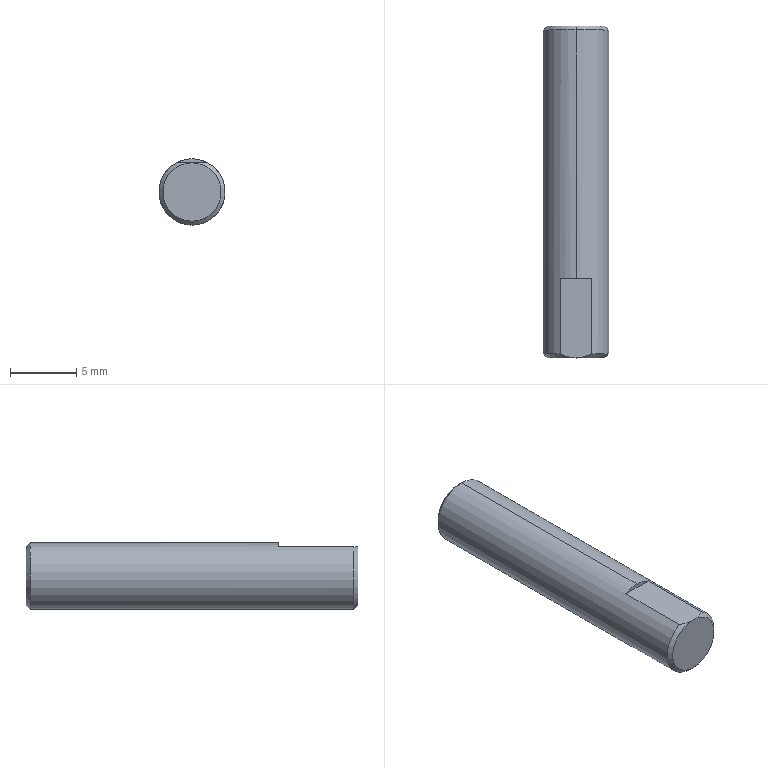Part | SolidWorks | features Chamfer 1, Extrusion 1, ICE 1 | 1 solid | 10 faces | box 5 x 25 x 5 mm | volume 486.718 mm3 | cone 4 | plane 4 | cylinder 2 | commonest cylinder face diameters 5 x2
STEP:
#1=CARTESIAN_POINT('',(0.,25.,2.2));
#2=VERTEX_POINT('',#1);
#3=CARTESIAN_POINT('',(0.,25.,-2.2));
#4=VERTEX_POINT('',#3);
#5=CARTESIAN_POINT('',(0.,25.,0.));
#6=DIRECTION('',(0.,1.,0.));
#7=DIRECTION('',(0.,0.,1.));
#8=AXIS2_PLACEMENT_3D('',#5,#6,#7);
#9=CIRCLE('',#8,2.2);
#10=EDGE_CURVE('',#2,#4,#9,.T.);
#11=ORIENTED_EDGE('',*,*,#10,.F.);
#12=CARTESIAN_POINT('',(0.,24.7,2.5));
#13=VERTEX_POINT('',#12);
#14=CARTESIAN_POINT('',(0.,25.,2.2));
#15=DIRECTION('',(0.,-0.7071,0.7071));
#16=VECTOR('',#15,1000.);
#17=LINE('',#14,#16);
#18=EDGE_CURVE('',#2,#13,#17,.T.);
#19=ORIENTED_EDGE('',*,*,#18,.T.);
#20=CARTESIAN_POINT('',(0.,24.7,-2.5));
#21=VERTEX_POINT('',#20);
#22=CARTESIAN_POINT('',(0.,24.7,0.));
#23=DIRECTION('',(0.,-1.,0.));
#24=DIRECTION('',(0.,0.,1.));
#25=AXIS2_PLACEMENT_3D('',#22,#23,#24);
#26=CIRCLE('',#25,2.5);
#27=EDGE_CURVE('',#21,#13,#26,.T.);
#28=ORIENTED_EDGE('',*,*,#27,.F.);
#29=CARTESIAN_POINT('',(0.,25.,-2.2));
#30=DIRECTION('',(0.,-0.7071,-0.7071));
#31=VECTOR('',#30,1000.);
#32=LINE('',#29,#31);
#33=EDGE_CURVE('',#4,#21,#32,.T.);
#34=ORIENTED_EDGE('',*,*,#33,.F.);
#35=EDGE_LOOP('',(#11,#19,#28,#34));
#36=FACE_OUTER_BOUND('',#35,.T.);
#37=CARTESIAN_POINT('',(0.,25.,0.));
#38=DIRECTION('',(0.,-1.,0.));
#39=DIRECTION('',(0.,0.,-1.));
#40=AXIS2_PLACEMENT_3D('',#37,#38,#39);
#41=CONICAL_SURFACE('',#40,2.2,0.7854);
#42=ADVANCED_FACE('',(#36),#41,.T.);
#43=CARTESIAN_POINT('',(0.,0.,-2.2));
#44=VERTEX_POINT('',#43);
#45=CARTESIAN_POINT('',(0.,0.,2.2));
#46=VERTEX_POINT('',#45);
#47=CARTESIAN_POINT('',(0.,0.,0.));
#48=DIRECTION('',(0.,-1.,0.));
#49=DIRECTION('',(0.,0.,1.));
#50=AXIS2_PLACEMENT_3D('',#47,#48,#49);
#51=CIRCLE('',#50,2.2);
#52=EDGE_CURVE('',#44,#46,#51,.T.);
#53=ORIENTED_EDGE('',*,*,#52,.F.);
#54=CARTESIAN_POINT('',(0.,0.3,-2.5));
#55=VERTEX_POINT('',#54);
#56=CARTESIAN_POINT('',(0.,0.3,-2.5));
#57=DIRECTION('',(0.,0.7071,-0.7071));
#58=VECTOR('',#57,1000.);
#59=LINE('',#56,#58);
#60=EDGE_CURVE('',#44,#55,#59,.T.);
#61=ORIENTED_EDGE('',*,*,#60,.T.);
#62=CARTESIAN_POINT('',(1.187,0.3,2.2));
#63=VERTEX_POINT('',#62);
#64=CARTESIAN_POINT('',(0.,0.3,0.));
#65=DIRECTION('',(0.,1.,0.));
#66=DIRECTION('',(0.,0.,1.));
#67=AXIS2_PLACEMENT_3D('',#64,#65,#66);
#68=CIRCLE('',#67,2.5);
#69=EDGE_CURVE('',#63,#55,#68,.T.);
#70=ORIENTED_EDGE('',*,*,#69,.F.);
#71=CARTESIAN_POINT('',(0.,0.,2.2));
#72=CARTESIAN_POINT('',(0.205,0.,2.2));
#73=CARTESIAN_POINT('',(0.4129,0.03019,2.2));
#74=CARTESIAN_POINT('',(0.8105,0.1367,2.2));
#75=CARTESIAN_POINT('',(1.001,0.2116,2.2));
#76=CARTESIAN_POINT('',(1.187,0.3,2.2));
#77=B_SPLINE_CURVE_WITH_KNOTS('',3,(#71,#72,#73,#74,#75,#76),.UNSPECIFIED.,.F.,.F.,(4,2,4),(0.004471,0.005085,0.005698),.UNSPECIFIED.);
#78=EDGE_CURVE('',#46,#63,#77,.T.);
#79=ORIENTED_EDGE('',*,*,#78,.F.);
#80=EDGE_LOOP('',(#53,#61,#70,#79));
#81=FACE_OUTER_BOUND('',#80,.T.);
#82=CARTESIAN_POINT('',(0.,0.3,0.));
#83=DIRECTION('',(0.,1.,0.));
#84=DIRECTION('',(0.,0.,1.));
#85=AXIS2_PLACEMENT_3D('',#82,#83,#84);
#86=CONICAL_SURFACE('',#85,2.5,0.7854);
#87=ADVANCED_FACE('',(#81),#86,.T.);
#88=ORIENTED_EDGE('',*,*,#27,.T.);
#89=CARTESIAN_POINT('',(0.,6.,2.5));
#90=VERTEX_POINT('',#89);
#91=CARTESIAN_POINT('',(0.,25.,2.5));
#92=DIRECTION('',(0.,-1.,0.));
#93=VECTOR('',#92,1000.);
#94=LINE('',#91,#93);
#95=EDGE_CURVE('',#13,#90,#94,.T.);
#96=ORIENTED_EDGE('',*,*,#95,.T.);
#97=CARTESIAN_POINT('',(1.187,6.,2.2));
#98=VERTEX_POINT('',#97);
#99=CARTESIAN_POINT('',(0.,6.,0.));
#100=DIRECTION('',(0.,-1.,0.));
#101=DIRECTION('',(0.,0.,-1.));
#102=AXIS2_PLACEMENT_3D('',#99,#100,#101);
#103=CIRCLE('',#102,2.5);
#104=EDGE_CURVE('',#98,#90,#103,.T.);
#105=ORIENTED_EDGE('',*,*,#104,.F.);
#106=CARTESIAN_POINT('',(1.187,25.,2.2));
#107=DIRECTION('',(0.,-1.,0.));
#108=VECTOR('',#107,1000.);
#109=LINE('',#106,#108);
#110=EDGE_CURVE('',#98,#63,#109,.T.);
#111=ORIENTED_EDGE('',*,*,#110,.T.);
#112=ORIENTED_EDGE('',*,*,#69,.T.);
#113=CARTESIAN_POINT('',(0.,25.,-2.5));
#114=DIRECTION('',(0.,-1.,0.));
#115=VECTOR('',#114,1000.);
#116=LINE('',#113,#115);
#117=EDGE_CURVE('',#21,#55,#116,.T.);
#118=ORIENTED_EDGE('',*,*,#117,.F.);
#119=EDGE_LOOP('',(#88,#96,#105,#111,#112,#118));
#120=FACE_OUTER_BOUND('',#119,.T.);
#121=CARTESIAN_POINT('',(0.,25.,0.));
#122=DIRECTION('',(0.,-1.,0.));
#123=DIRECTION('',(0.,0.,-1.));
#124=AXIS2_PLACEMENT_3D('',#121,#122,#123);
#125=CYLINDRICAL_SURFACE('',#124,2.5);
#126=ADVANCED_FACE('',(#120),#125,.T.);
#127=ORIENTED_EDGE('',*,*,#95,.F.);
#128=CARTESIAN_POINT('',(0.,24.7,0.));
#129=DIRECTION('',(0.,-1.,0.));
#130=DIRECTION('',(0.,0.,1.));
#131=AXIS2_PLACEMENT_3D('',#128,#129,#130);
#132=CIRCLE('',#131,2.5);
#133=EDGE_CURVE('',#13,#21,#132,.T.);
#134=ORIENTED_EDGE('',*,*,#133,.T.);
#135=ORIENTED_EDGE('',*,*,#117,.T.);
#136=CARTESIAN_POINT('',(-1.187,0.3,2.2));
#137=VERTEX_POINT('',#136);
#138=CARTESIAN_POINT('',(0.,0.3,0.));
#139=DIRECTION('',(0.,1.,0.));
#140=DIRECTION('',(0.,0.,1.));
#141=AXIS2_PLACEMENT_3D('',#138,#139,#140);
#142=CIRCLE('',#141,2.5);
#143=EDGE_CURVE('',#55,#137,#142,.T.);
#144=ORIENTED_EDGE('',*,*,#143,.T.);
#145=CARTESIAN_POINT('',(-1.187,6.,2.2));
#146=VERTEX_POINT('',#145);
#147=CARTESIAN_POINT('',(-1.187,25.,2.2));
#148=DIRECTION('',(0.,1.,0.));
#149=VECTOR('',#148,1000.);
#150=LINE('',#147,#149);
#151=EDGE_CURVE('',#137,#146,#150,.T.);
#152=ORIENTED_EDGE('',*,*,#151,.T.);
#153=CARTESIAN_POINT('',(0.,6.,0.));
#154=DIRECTION('',(0.,-1.,0.));
#155=DIRECTION('',(0.,0.,-1.));
#156=AXIS2_PLACEMENT_3D('',#153,#154,#155);
#157=CIRCLE('',#156,2.5);
#158=EDGE_CURVE('',#90,#146,#157,.T.);
#159=ORIENTED_EDGE('',*,*,#158,.F.);
#160=EDGE_LOOP('',(#127,#134,#135,#144,#152,#159));
#161=FACE_OUTER_BOUND('',#160,.T.);
#162=CARTESIAN_POINT('',(0.,25.,0.));
#163=DIRECTION('',(0.,-1.,0.));
#164=DIRECTION('',(0.,0.,-1.));
#165=AXIS2_PLACEMENT_3D('',#162,#163,#164);
#166=CYLINDRICAL_SURFACE('',#165,2.5);
#167=ADVANCED_FACE('',(#161),#166,.T.);
#168=CARTESIAN_POINT('',(0.,25.,0.));
#169=DIRECTION('',(0.,1.,0.));
#170=DIRECTION('',(0.,0.,1.));
#171=AXIS2_PLACEMENT_3D('',#168,#169,#170);
#172=CIRCLE('',#171,2.2);
#173=EDGE_CURVE('',#4,#2,#172,.T.);
#174=ORIENTED_EDGE('',*,*,#173,.T.);
#175=ORIENTED_EDGE('',*,*,#10,.T.);
#176=EDGE_LOOP('',(#174,#175));
#177=FACE_OUTER_BOUND('',#176,.T.);
#178=CARTESIAN_POINT('',(0.,25.,0.));
#179=DIRECTION('',(0.,1.,0.));
#180=DIRECTION('',(0.,0.,1.));
#181=AXIS2_PLACEMENT_3D('',#178,#179,#180);
#182=PLANE('',#181);
#183=ADVANCED_FACE('',(#177),#182,.T.);
#184=CARTESIAN_POINT('',(0.,0.,0.));
#185=DIRECTION('',(0.,-1.,0.));
#186=DIRECTION('',(0.,0.,1.));
#187=AXIS2_PLACEMENT_3D('',#184,#185,#186);
#188=CIRCLE('',#187,2.2);
#189=EDGE_CURVE('',#46,#44,#188,.T.);
#190=ORIENTED_EDGE('',*,*,#189,.T.);
#191=ORIENTED_EDGE('',*,*,#52,.T.);
#192=EDGE_LOOP('',(#190,#191));
#193=FACE_OUTER_BOUND('',#192,.T.);
#194=CARTESIAN_POINT('',(0.,0.,0.));
#195=DIRECTION('',(0.,1.,0.));
#196=DIRECTION('',(0.,0.,1.));
#197=AXIS2_PLACEMENT_3D('',#194,#195,#196);
#198=PLANE('',#197);
#199=ADVANCED_FACE('',(#193),#198,.F.);
#200=ORIENTED_EDGE('',*,*,#60,.F.);
#201=ORIENTED_EDGE('',*,*,#189,.F.);
#202=CARTESIAN_POINT('',(-1.187,0.3,2.2));
#203=CARTESIAN_POINT('',(-1.001,0.2117,2.2));
#204=CARTESIAN_POINT('',(-0.8106,0.1367,2.2));
#205=CARTESIAN_POINT('',(-0.413,0.03021,2.2));
#206=CARTESIAN_POINT('',(-0.2051,0.,2.2));
#207=CARTESIAN_POINT('',(0.,0.,2.2));
#208=B_SPLINE_CURVE_WITH_KNOTS('',3,(#202,#203,#204,#205,#206,#207),.UNSPECIFIED.,.F.,.F.,(4,2,4),(0.003244,0.003858,0.004471),.UNSPECIFIED.);
#209=EDGE_CURVE('',#137,#46,#208,.T.);
#210=ORIENTED_EDGE('',*,*,#209,.F.);
#211=ORIENTED_EDGE('',*,*,#143,.F.);
#212=EDGE_LOOP('',(#200,#201,#210,#211));
#213=FACE_OUTER_BOUND('',#212,.T.);
#214=CARTESIAN_POINT('',(0.,0.3,0.));
#215=DIRECTION('',(0.,1.,0.));
#216=DIRECTION('',(0.,0.,1.));
#217=AXIS2_PLACEMENT_3D('',#214,#215,#216);
#218=CONICAL_SURFACE('',#217,2.5,0.7854);
#219=ADVANCED_FACE('',(#213),#218,.T.);
#220=ORIENTED_EDGE('',*,*,#18,.F.);
#221=ORIENTED_EDGE('',*,*,#173,.F.);
#222=ORIENTED_EDGE('',*,*,#33,.T.);
#223=ORIENTED_EDGE('',*,*,#133,.F.);
#224=EDGE_LOOP('',(#220,#221,#222,#223));
#225=FACE_OUTER_BOUND('',#224,.T.);
#226=CARTESIAN_POINT('',(0.,25.,0.));
#227=DIRECTION('',(0.,-1.,0.));
#228=DIRECTION('',(0.,0.,-1.));
#229=AXIS2_PLACEMENT_3D('',#226,#227,#228);
#230=CONICAL_SURFACE('',#229,2.2,0.7854);
#231=ADVANCED_FACE('',(#225),#230,.T.);
#232=ORIENTED_EDGE('',*,*,#104,.T.);
#233=ORIENTED_EDGE('',*,*,#158,.T.);
#234=CARTESIAN_POINT('',(-2.016,6.,2.2));
#235=DIRECTION('',(1.,0.,0.));
#236=VECTOR('',#235,1000.);
#237=LINE('',#234,#236);
#238=EDGE_CURVE('',#146,#98,#237,.T.);
#239=ORIENTED_EDGE('',*,*,#238,.T.);
#240=EDGE_LOOP('',(#232,#233,#239));
#241=FACE_OUTER_BOUND('',#240,.T.);
#242=CARTESIAN_POINT('',(0.,6.,0.));
#243=DIRECTION('',(0.,-1.,0.));
#244=DIRECTION('',(0.,0.,-1.));
#245=AXIS2_PLACEMENT_3D('',#242,#243,#244);
#246=PLANE('',#245);
#247=ADVANCED_FACE('',(#241),#246,.T.);
#248=ORIENTED_EDGE('',*,*,#238,.F.);
#249=ORIENTED_EDGE('',*,*,#151,.F.);
#250=ORIENTED_EDGE('',*,*,#209,.T.);
#251=ORIENTED_EDGE('',*,*,#78,.T.);
#252=ORIENTED_EDGE('',*,*,#110,.F.);
#253=EDGE_LOOP('',(#248,#249,#250,#251,#252));
#254=FACE_OUTER_BOUND('',#253,.T.);
#255=CARTESIAN_POINT('',(-2.016,6.,2.2));
#256=DIRECTION('',(0.,0.,-1.));
#257=DIRECTION('',(-1.,0.,0.));
#258=AXIS2_PLACEMENT_3D('',#255,#256,#257);
#259=PLANE('',#258);
#260=ADVANCED_FACE('',(#254),#259,.F.);
#261=CLOSED_SHELL('',(#42,#87,#126,#167,#183,#199,#219,#231,#247,#260));
#262=MANIFOLD_SOLID_BREP('',#261);
#263=CARTESIAN_POINT('',(0.,0.,0.));
#264=DIRECTION('',(0.,0.,1.));
#265=DIRECTION('',(1.,0.,0.));
#266=AXIS2_PLACEMENT_3D('',#263,#264,#265);
#267=(LENGTH_UNIT()NAMED_UNIT(*)SI_UNIT(.MILLI.,.METRE.));
#268=UNCERTAINTY_MEASURE_WITH_UNIT(LENGTH_MEASURE(0.00001),#267,'','');
#269=(NAMED_UNIT(*)PLANE_ANGLE_UNIT()SI_UNIT($,.RADIAN.));
#270=(NAMED_UNIT(*)SI_UNIT($,.STERADIAN.)SOLID_ANGLE_UNIT());
#271=(GEOMETRIC_REPRESENTATION_CONTEXT(3)GLOBAL_UNCERTAINTY_ASSIGNED_CONTEXT((#268))GLOBAL_UNIT_ASSIGNED_CONTEXT((#267,#269,#270))REPRESENTATION_CONTEXT('',''));
#272=ADVANCED_BREP_SHAPE_REPRESENTATION('',(#262,#266),#271);